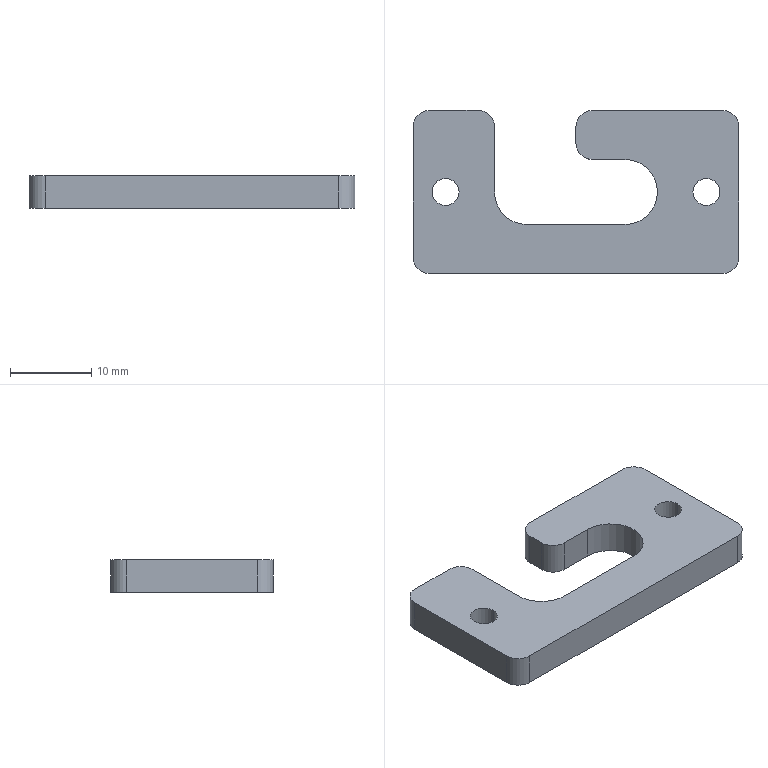Part | SolidWorks | features BreakCorner 1, FlatPattern 1, HoleWzd 1, ICE 1, SMBaseFlange 1, SheetMetal 1 | 1 solid | 24 faces | box 40 x 20 x 4 mm | volume 2269 mm3 | cylinder 13 | plane 11 | commonest cylinder face diameters 4 x7 3.3 x4 8 x2
STEP:
#1=CARTESIAN_POINT('',(-17.65,0.,-4.));
#2=VERTEX_POINT('',#1);
#3=CARTESIAN_POINT('',(-14.35,0.,-4.));
#4=VERTEX_POINT('',#3);
#5=CARTESIAN_POINT('',(-16.,0.,-4.));
#6=DIRECTION('',(0.,0.,1.));
#7=DIRECTION('',(1.,0.,0.));
#8=AXIS2_PLACEMENT_3D('',#5,#6,#7);
#9=CIRCLE('',#8,1.65);
#10=EDGE_CURVE('',#2,#4,#9,.T.);
#11=ORIENTED_EDGE('',*,*,#10,.F.);
#12=CARTESIAN_POINT('',(-17.65,0.,0.));
#13=VERTEX_POINT('',#12);
#14=CARTESIAN_POINT('',(-17.65,0.,0.));
#15=DIRECTION('',(0.,0.,1.));
#16=VECTOR('',#15,1000.);
#17=LINE('',#14,#16);
#18=EDGE_CURVE('',#2,#13,#17,.T.);
#19=ORIENTED_EDGE('',*,*,#18,.T.);
#20=CARTESIAN_POINT('',(-14.35,0.,0.));
#21=VERTEX_POINT('',#20);
#22=CARTESIAN_POINT('',(-16.,0.,0.));
#23=DIRECTION('',(0.,0.,1.));
#24=DIRECTION('',(1.,0.,0.));
#25=AXIS2_PLACEMENT_3D('',#22,#23,#24);
#26=CIRCLE('',#25,1.65);
#27=EDGE_CURVE('',#13,#21,#26,.T.);
#28=ORIENTED_EDGE('',*,*,#27,.T.);
#29=CARTESIAN_POINT('',(-14.35,0.,0.));
#30=DIRECTION('',(0.,0.,1.));
#31=VECTOR('',#30,1000.);
#32=LINE('',#29,#31);
#33=EDGE_CURVE('',#4,#21,#32,.T.);
#34=ORIENTED_EDGE('',*,*,#33,.F.);
#35=EDGE_LOOP('',(#11,#19,#28,#34));
#36=FACE_OUTER_BOUND('',#35,.T.);
#37=CARTESIAN_POINT('',(-16.,0.,0.));
#38=DIRECTION('',(0.,0.,1.));
#39=DIRECTION('',(1.,0.,0.));
#40=AXIS2_PLACEMENT_3D('',#37,#38,#39);
#41=CYLINDRICAL_SURFACE('',#40,1.65);
#42=ADVANCED_FACE('',(#36),#41,.F.);
#43=CARTESIAN_POINT('',(14.35,0.,-4.));
#44=VERTEX_POINT('',#43);
#45=CARTESIAN_POINT('',(17.65,0.,-4.));
#46=VERTEX_POINT('',#45);
#47=CARTESIAN_POINT('',(16.,0.,-4.));
#48=DIRECTION('',(0.,0.,1.));
#49=DIRECTION('',(1.,0.,0.));
#50=AXIS2_PLACEMENT_3D('',#47,#48,#49);
#51=CIRCLE('',#50,1.65);
#52=EDGE_CURVE('',#44,#46,#51,.T.);
#53=ORIENTED_EDGE('',*,*,#52,.F.);
#54=CARTESIAN_POINT('',(14.35,0.,0.));
#55=VERTEX_POINT('',#54);
#56=CARTESIAN_POINT('',(14.35,0.,0.));
#57=DIRECTION('',(0.,0.,1.));
#58=VECTOR('',#57,1000.);
#59=LINE('',#56,#58);
#60=EDGE_CURVE('',#44,#55,#59,.T.);
#61=ORIENTED_EDGE('',*,*,#60,.T.);
#62=CARTESIAN_POINT('',(17.65,0.,0.));
#63=VERTEX_POINT('',#62);
#64=CARTESIAN_POINT('',(16.,0.,0.));
#65=DIRECTION('',(0.,0.,1.));
#66=DIRECTION('',(1.,0.,0.));
#67=AXIS2_PLACEMENT_3D('',#64,#65,#66);
#68=CIRCLE('',#67,1.65);
#69=EDGE_CURVE('',#55,#63,#68,.T.);
#70=ORIENTED_EDGE('',*,*,#69,.T.);
#71=CARTESIAN_POINT('',(17.65,0.,0.));
#72=DIRECTION('',(0.,0.,1.));
#73=VECTOR('',#72,1000.);
#74=LINE('',#71,#73);
#75=EDGE_CURVE('',#46,#63,#74,.T.);
#76=ORIENTED_EDGE('',*,*,#75,.F.);
#77=EDGE_LOOP('',(#53,#61,#70,#76));
#78=FACE_OUTER_BOUND('',#77,.T.);
#79=CARTESIAN_POINT('',(16.,0.,0.));
#80=DIRECTION('',(0.,0.,1.));
#81=DIRECTION('',(1.,0.,0.));
#82=AXIS2_PLACEMENT_3D('',#79,#80,#81);
#83=CYLINDRICAL_SURFACE('',#82,1.65);
#84=ADVANCED_FACE('',(#78),#83,.F.);
#85=CARTESIAN_POINT('',(-12.,10.,-4.));
#86=VERTEX_POINT('',#85);
#87=CARTESIAN_POINT('',(-18.,10.,-4.));
#88=VERTEX_POINT('',#87);
#89=CARTESIAN_POINT('',(-20.,10.,-4.));
#90=DIRECTION('',(-1.,0.,0.));
#91=VECTOR('',#90,1000.);
#92=LINE('',#89,#91);
#93=EDGE_CURVE('',#86,#88,#92,.T.);
#94=ORIENTED_EDGE('',*,*,#93,.T.);
#95=CARTESIAN_POINT('',(-18.,10.,0.));
#96=VERTEX_POINT('',#95);
#97=CARTESIAN_POINT('',(-18.,10.,-4.));
#98=DIRECTION('',(0.,0.,1.));
#99=VECTOR('',#98,1000.);
#100=LINE('',#97,#99);
#101=EDGE_CURVE('',#88,#96,#100,.T.);
#102=ORIENTED_EDGE('',*,*,#101,.T.);
#103=CARTESIAN_POINT('',(-12.,10.,0.));
#104=VERTEX_POINT('',#103);
#105=CARTESIAN_POINT('',(-20.,10.,0.));
#106=DIRECTION('',(-1.,0.,0.));
#107=VECTOR('',#106,1000.);
#108=LINE('',#105,#107);
#109=EDGE_CURVE('',#104,#96,#108,.T.);
#110=ORIENTED_EDGE('',*,*,#109,.F.);
#111=CARTESIAN_POINT('',(-12.,10.,-4.));
#112=DIRECTION('',(0.,0.,-1.));
#113=VECTOR('',#112,1000.);
#114=LINE('',#111,#113);
#115=EDGE_CURVE('',#104,#86,#114,.T.);
#116=ORIENTED_EDGE('',*,*,#115,.T.);
#117=EDGE_LOOP('',(#94,#102,#110,#116));
#118=FACE_OUTER_BOUND('',#117,.T.);
#119=CARTESIAN_POINT('',(-20.,10.,-4.));
#120=DIRECTION('',(0.,1.,0.));
#121=DIRECTION('',(0.,0.,1.));
#122=AXIS2_PLACEMENT_3D('',#119,#120,#121);
#123=PLANE('',#122);
#124=ADVANCED_FACE('',(#118),#123,.T.);
#125=CARTESIAN_POINT('',(20.,-8.,-4.));
#126=VERTEX_POINT('',#125);
#127=CARTESIAN_POINT('',(20.,8.,-4.));
#128=VERTEX_POINT('',#127);
#129=CARTESIAN_POINT('',(20.,10.,-4.));
#130=DIRECTION('',(0.,1.,0.));
#131=VECTOR('',#130,1000.);
#132=LINE('',#129,#131);
#133=EDGE_CURVE('',#126,#128,#132,.T.);
#134=ORIENTED_EDGE('',*,*,#133,.T.);
#135=CARTESIAN_POINT('',(20.,8.,0.));
#136=VERTEX_POINT('',#135);
#137=CARTESIAN_POINT('',(20.,8.,-4.));
#138=DIRECTION('',(0.,0.,1.));
#139=VECTOR('',#138,1000.);
#140=LINE('',#137,#139);
#141=EDGE_CURVE('',#128,#136,#140,.T.);
#142=ORIENTED_EDGE('',*,*,#141,.T.);
#143=CARTESIAN_POINT('',(20.,-8.,0.));
#144=VERTEX_POINT('',#143);
#145=CARTESIAN_POINT('',(20.,10.,0.));
#146=DIRECTION('',(0.,1.,0.));
#147=VECTOR('',#146,1000.);
#148=LINE('',#145,#147);
#149=EDGE_CURVE('',#144,#136,#148,.T.);
#150=ORIENTED_EDGE('',*,*,#149,.F.);
#151=CARTESIAN_POINT('',(20.,-8.,-4.));
#152=DIRECTION('',(0.,0.,-1.));
#153=VECTOR('',#152,1000.);
#154=LINE('',#151,#153);
#155=EDGE_CURVE('',#144,#126,#154,.T.);
#156=ORIENTED_EDGE('',*,*,#155,.T.);
#157=EDGE_LOOP('',(#134,#142,#150,#156));
#158=FACE_OUTER_BOUND('',#157,.T.);
#159=CARTESIAN_POINT('',(20.,10.,-4.));
#160=DIRECTION('',(1.,0.,0.));
#161=DIRECTION('',(0.,1.,0.));
#162=AXIS2_PLACEMENT_3D('',#159,#160,#161);
#163=PLANE('',#162);
#164=ADVANCED_FACE('',(#158),#163,.T.);
#165=CARTESIAN_POINT('',(-18.,-10.,-4.));
#166=VERTEX_POINT('',#165);
#167=CARTESIAN_POINT('',(18.,-10.,-4.));
#168=VERTEX_POINT('',#167);
#169=CARTESIAN_POINT('',(-20.,-10.,-4.));
#170=DIRECTION('',(1.,0.,0.));
#171=VECTOR('',#170,1000.);
#172=LINE('',#169,#171);
#173=EDGE_CURVE('',#166,#168,#172,.T.);
#174=ORIENTED_EDGE('',*,*,#173,.T.);
#175=CARTESIAN_POINT('',(18.,-10.,0.));
#176=VERTEX_POINT('',#175);
#177=CARTESIAN_POINT('',(18.,-10.,-4.));
#178=DIRECTION('',(0.,0.,1.));
#179=VECTOR('',#178,1000.);
#180=LINE('',#177,#179);
#181=EDGE_CURVE('',#168,#176,#180,.T.);
#182=ORIENTED_EDGE('',*,*,#181,.T.);
#183=CARTESIAN_POINT('',(-18.,-10.,0.));
#184=VERTEX_POINT('',#183);
#185=CARTESIAN_POINT('',(-20.,-10.,0.));
#186=DIRECTION('',(1.,0.,0.));
#187=VECTOR('',#186,1000.);
#188=LINE('',#185,#187);
#189=EDGE_CURVE('',#184,#176,#188,.T.);
#190=ORIENTED_EDGE('',*,*,#189,.F.);
#191=CARTESIAN_POINT('',(-18.,-10.,-4.));
#192=DIRECTION('',(0.,0.,-1.));
#193=VECTOR('',#192,1000.);
#194=LINE('',#191,#193);
#195=EDGE_CURVE('',#184,#166,#194,.T.);
#196=ORIENTED_EDGE('',*,*,#195,.T.);
#197=EDGE_LOOP('',(#174,#182,#190,#196));
#198=FACE_OUTER_BOUND('',#197,.T.);
#199=CARTESIAN_POINT('',(-20.,-10.,-4.));
#200=DIRECTION('',(0.,-1.,0.));
#201=DIRECTION('',(0.,0.,-1.));
#202=AXIS2_PLACEMENT_3D('',#199,#200,#201);
#203=PLANE('',#202);
#204=ADVANCED_FACE('',(#198),#203,.T.);
#205=CARTESIAN_POINT('',(-20.,8.,-4.));
#206=VERTEX_POINT('',#205);
#207=CARTESIAN_POINT('',(-20.,-8.,-4.));
#208=VERTEX_POINT('',#207);
#209=CARTESIAN_POINT('',(-20.,10.,-4.));
#210=DIRECTION('',(0.,-1.,0.));
#211=VECTOR('',#210,1000.);
#212=LINE('',#209,#211);
#213=EDGE_CURVE('',#206,#208,#212,.T.);
#214=ORIENTED_EDGE('',*,*,#213,.T.);
#215=CARTESIAN_POINT('',(-20.,-8.,0.));
#216=VERTEX_POINT('',#215);
#217=CARTESIAN_POINT('',(-20.,-8.,-4.));
#218=DIRECTION('',(0.,0.,1.));
#219=VECTOR('',#218,1000.);
#220=LINE('',#217,#219);
#221=EDGE_CURVE('',#208,#216,#220,.T.);
#222=ORIENTED_EDGE('',*,*,#221,.T.);
#223=CARTESIAN_POINT('',(-20.,8.,0.));
#224=VERTEX_POINT('',#223);
#225=CARTESIAN_POINT('',(-20.,10.,0.));
#226=DIRECTION('',(0.,-1.,0.));
#227=VECTOR('',#226,1000.);
#228=LINE('',#225,#227);
#229=EDGE_CURVE('',#224,#216,#228,.T.);
#230=ORIENTED_EDGE('',*,*,#229,.F.);
#231=CARTESIAN_POINT('',(-20.,8.,-4.));
#232=DIRECTION('',(0.,0.,-1.));
#233=VECTOR('',#232,1000.);
#234=LINE('',#231,#233);
#235=EDGE_CURVE('',#224,#206,#234,.T.);
#236=ORIENTED_EDGE('',*,*,#235,.T.);
#237=EDGE_LOOP('',(#214,#222,#230,#236));
#238=FACE_OUTER_BOUND('',#237,.T.);
#239=CARTESIAN_POINT('',(-20.,10.,-4.));
#240=DIRECTION('',(-1.,0.,0.));
#241=DIRECTION('',(0.,0.,1.));
#242=AXIS2_PLACEMENT_3D('',#239,#240,#241);
#243=PLANE('',#242);
#244=ADVANCED_FACE('',(#238),#243,.T.);
#245=CARTESIAN_POINT('',(18.,10.,-4.));
#246=VERTEX_POINT('',#245);
#247=CARTESIAN_POINT('',(2.,10.,-4.));
#248=VERTEX_POINT('',#247);
#249=CARTESIAN_POINT('',(-20.,10.,-4.));
#250=DIRECTION('',(-1.,0.,0.));
#251=VECTOR('',#250,1000.);
#252=LINE('',#249,#251);
#253=EDGE_CURVE('',#246,#248,#252,.T.);
#254=ORIENTED_EDGE('',*,*,#253,.T.);
#255=CARTESIAN_POINT('',(2.,10.,0.));
#256=VERTEX_POINT('',#255);
#257=CARTESIAN_POINT('',(2.,10.,0.));
#258=DIRECTION('',(0.,0.,1.));
#259=VECTOR('',#258,1000.);
#260=LINE('',#257,#259);
#261=EDGE_CURVE('',#248,#256,#260,.T.);
#262=ORIENTED_EDGE('',*,*,#261,.T.);
#263=CARTESIAN_POINT('',(18.,10.,0.));
#264=VERTEX_POINT('',#263);
#265=CARTESIAN_POINT('',(-20.,10.,0.));
#266=DIRECTION('',(-1.,0.,0.));
#267=VECTOR('',#266,1000.);
#268=LINE('',#265,#267);
#269=EDGE_CURVE('',#264,#256,#268,.T.);
#270=ORIENTED_EDGE('',*,*,#269,.F.);
#271=CARTESIAN_POINT('',(18.,10.,-4.));
#272=DIRECTION('',(0.,0.,-1.));
#273=VECTOR('',#272,1000.);
#274=LINE('',#271,#273);
#275=EDGE_CURVE('',#264,#246,#274,.T.);
#276=ORIENTED_EDGE('',*,*,#275,.T.);
#277=EDGE_LOOP('',(#254,#262,#270,#276));
#278=FACE_OUTER_BOUND('',#277,.T.);
#279=CARTESIAN_POINT('',(-20.,10.,-4.));
#280=DIRECTION('',(0.,1.,0.));
#281=DIRECTION('',(0.,0.,1.));
#282=AXIS2_PLACEMENT_3D('',#279,#280,#281);
#283=PLANE('',#282);
#284=ADVANCED_FACE('',(#278),#283,.T.);
#285=CARTESIAN_POINT('',(-16.,0.,-4.));
#286=DIRECTION('',(0.,0.,1.));
#287=DIRECTION('',(1.,0.,0.));
#288=AXIS2_PLACEMENT_3D('',#285,#286,#287);
#289=CIRCLE('',#288,1.65);
#290=EDGE_CURVE('',#4,#2,#289,.T.);
#291=ORIENTED_EDGE('',*,*,#290,.T.);
#292=ORIENTED_EDGE('',*,*,#10,.T.);
#293=EDGE_LOOP('',(#291,#292));
#294=FACE_BOUND('',#293,.T.);
#295=CARTESIAN_POINT('',(16.,0.,-4.));
#296=DIRECTION('',(0.,0.,1.));
#297=DIRECTION('',(1.,0.,0.));
#298=AXIS2_PLACEMENT_3D('',#295,#296,#297);
#299=CIRCLE('',#298,1.65);
#300=EDGE_CURVE('',#46,#44,#299,.T.);
#301=ORIENTED_EDGE('',*,*,#300,.T.);
#302=ORIENTED_EDGE('',*,*,#52,.T.);
#303=EDGE_LOOP('',(#301,#302));
#304=FACE_BOUND('',#303,.T.);
#305=CARTESIAN_POINT('',(6.,4.,-4.));
#306=VERTEX_POINT('',#305);
#307=CARTESIAN_POINT('',(2.,4.,-4.));
#308=VERTEX_POINT('',#307);
#309=CARTESIAN_POINT('',(0.,4.,-4.));
#310=DIRECTION('',(-1.,0.,0.));
#311=VECTOR('',#310,1000.);
#312=LINE('',#309,#311);
#313=EDGE_CURVE('',#306,#308,#312,.T.);
#314=ORIENTED_EDGE('',*,*,#313,.T.);
#315=CARTESIAN_POINT('',(0.,6.,-4.));
#316=VERTEX_POINT('',#315);
#317=CARTESIAN_POINT('',(2.,6.,-4.));
#318=DIRECTION('',(0.,0.,-1.));
#319=DIRECTION('',(1.,0.,0.));
#320=AXIS2_PLACEMENT_3D('',#317,#318,#319);
#321=CIRCLE('',#320,2.);
#322=EDGE_CURVE('',#308,#316,#321,.T.);
#323=ORIENTED_EDGE('',*,*,#322,.T.);
#324=CARTESIAN_POINT('',(0.,8.,-4.));
#325=VERTEX_POINT('',#324);
#326=CARTESIAN_POINT('',(0.,0.,-4.));
#327=DIRECTION('',(0.,1.,0.));
#328=VECTOR('',#327,1000.);
#329=LINE('',#326,#328);
#330=EDGE_CURVE('',#316,#325,#329,.T.);
#331=ORIENTED_EDGE('',*,*,#330,.T.);
#332=CARTESIAN_POINT('',(2.,8.,-4.));
#333=DIRECTION('',(0.,0.,-1.));
#334=DIRECTION('',(1.,0.,0.));
#335=AXIS2_PLACEMENT_3D('',#332,#333,#334);
#336=CIRCLE('',#335,2.);
#337=EDGE_CURVE('',#325,#248,#336,.T.);
#338=ORIENTED_EDGE('',*,*,#337,.T.);
#339=ORIENTED_EDGE('',*,*,#253,.F.);
#340=CARTESIAN_POINT('',(18.,8.,-4.));
#341=DIRECTION('',(0.,0.,-1.));
#342=DIRECTION('',(1.,0.,0.));
#343=AXIS2_PLACEMENT_3D('',#340,#341,#342);
#344=CIRCLE('',#343,2.);
#345=EDGE_CURVE('',#246,#128,#344,.T.);
#346=ORIENTED_EDGE('',*,*,#345,.T.);
#347=ORIENTED_EDGE('',*,*,#133,.F.);
#348=CARTESIAN_POINT('',(18.,-8.,-4.));
#349=DIRECTION('',(0.,0.,-1.));
#350=DIRECTION('',(1.,0.,0.));
#351=AXIS2_PLACEMENT_3D('',#348,#349,#350);
#352=CIRCLE('',#351,2.);
#353=EDGE_CURVE('',#126,#168,#352,.T.);
#354=ORIENTED_EDGE('',*,*,#353,.T.);
#355=ORIENTED_EDGE('',*,*,#173,.F.);
#356=CARTESIAN_POINT('',(-18.,-8.,-4.));
#357=DIRECTION('',(0.,0.,-1.));
#358=DIRECTION('',(1.,0.,0.));
#359=AXIS2_PLACEMENT_3D('',#356,#357,#358);
#360=CIRCLE('',#359,2.);
#361=EDGE_CURVE('',#166,#208,#360,.T.);
#362=ORIENTED_EDGE('',*,*,#361,.T.);
#363=ORIENTED_EDGE('',*,*,#213,.F.);
#364=CARTESIAN_POINT('',(-18.,8.,-4.));
#365=DIRECTION('',(0.,0.,-1.));
#366=DIRECTION('',(1.,0.,0.));
#367=AXIS2_PLACEMENT_3D('',#364,#365,#366);
#368=CIRCLE('',#367,2.);
#369=EDGE_CURVE('',#206,#88,#368,.T.);
#370=ORIENTED_EDGE('',*,*,#369,.T.);
#371=ORIENTED_EDGE('',*,*,#93,.F.);
#372=CARTESIAN_POINT('',(-10.,8.,-4.));
#373=VERTEX_POINT('',#372);
#374=CARTESIAN_POINT('',(-12.,8.,-4.));
#375=DIRECTION('',(0.,0.,-1.));
#376=DIRECTION('',(1.,0.,0.));
#377=AXIS2_PLACEMENT_3D('',#374,#375,#376);
#378=CIRCLE('',#377,2.);
#379=EDGE_CURVE('',#86,#373,#378,.T.);
#380=ORIENTED_EDGE('',*,*,#379,.T.);
#381=CARTESIAN_POINT('',(-10.,0.,-4.));
#382=VERTEX_POINT('',#381);
#383=CARTESIAN_POINT('',(-10.,0.,-4.));
#384=DIRECTION('',(0.,-1.,0.));
#385=VECTOR('',#384,1000.);
#386=LINE('',#383,#385);
#387=EDGE_CURVE('',#373,#382,#386,.T.);
#388=ORIENTED_EDGE('',*,*,#387,.T.);
#389=CARTESIAN_POINT('',(-6.,-4.,-4.));
#390=VERTEX_POINT('',#389);
#391=CARTESIAN_POINT('',(-6.,0.,-4.));
#392=DIRECTION('',(0.,0.,1.));
#393=DIRECTION('',(1.,0.,0.));
#394=AXIS2_PLACEMENT_3D('',#391,#392,#393);
#395=CIRCLE('',#394,4.);
#396=EDGE_CURVE('',#382,#390,#395,.T.);
#397=ORIENTED_EDGE('',*,*,#396,.T.);
#398=CARTESIAN_POINT('',(6.,-4.,-4.));
#399=VERTEX_POINT('',#398);
#400=CARTESIAN_POINT('',(0.,-4.,-4.));
#401=DIRECTION('',(1.,0.,0.));
#402=VECTOR('',#401,1000.);
#403=LINE('',#400,#402);
#404=EDGE_CURVE('',#390,#399,#403,.T.);
#405=ORIENTED_EDGE('',*,*,#404,.T.);
#406=CARTESIAN_POINT('',(6.,0.,-4.));
#407=DIRECTION('',(0.,0.,1.));
#408=DIRECTION('',(1.,0.,0.));
#409=AXIS2_PLACEMENT_3D('',#406,#407,#408);
#410=CIRCLE('',#409,4.);
#411=EDGE_CURVE('',#399,#306,#410,.T.);
#412=ORIENTED_EDGE('',*,*,#411,.T.);
#413=EDGE_LOOP('',(#314,#323,#331,#338,#339,#346,#347,#354,#355,#362,#363,#370,#371,#380,#388,#397,#405,#412));
#414=FACE_OUTER_BOUND('',#413,.T.);
#415=CARTESIAN_POINT('',(0.,0.,-4.));
#416=DIRECTION('',(0.,0.,1.));
#417=DIRECTION('',(1.,0.,0.));
#418=AXIS2_PLACEMENT_3D('',#415,#416,#417);
#419=PLANE('',#418);
#420=ADVANCED_FACE('',(#294,#304,#414),#419,.F.);
#421=CARTESIAN_POINT('',(-16.,0.,0.));
#422=DIRECTION('',(0.,0.,1.));
#423=DIRECTION('',(1.,0.,0.));
#424=AXIS2_PLACEMENT_3D('',#421,#422,#423);
#425=CIRCLE('',#424,1.65);
#426=EDGE_CURVE('',#21,#13,#425,.T.);
#427=ORIENTED_EDGE('',*,*,#426,.F.);
#428=ORIENTED_EDGE('',*,*,#27,.F.);
#429=EDGE_LOOP('',(#427,#428));
#430=FACE_BOUND('',#429,.T.);
#431=CARTESIAN_POINT('',(16.,0.,0.));
#432=DIRECTION('',(0.,0.,1.));
#433=DIRECTION('',(1.,0.,0.));
#434=AXIS2_PLACEMENT_3D('',#431,#432,#433);
#435=CIRCLE('',#434,1.65);
#436=EDGE_CURVE('',#63,#55,#435,.T.);
#437=ORIENTED_EDGE('',*,*,#436,.F.);
#438=ORIENTED_EDGE('',*,*,#69,.F.);
#439=EDGE_LOOP('',(#437,#438));
#440=FACE_BOUND('',#439,.T.);
#441=CARTESIAN_POINT('',(0.,6.,0.));
#442=VERTEX_POINT('',#441);
#443=CARTESIAN_POINT('',(0.,8.,0.));
#444=VERTEX_POINT('',#443);
#445=CARTESIAN_POINT('',(0.,0.,0.));
#446=DIRECTION('',(0.,1.,0.));
#447=VECTOR('',#446,1000.);
#448=LINE('',#445,#447);
#449=EDGE_CURVE('',#442,#444,#448,.T.);
#450=ORIENTED_EDGE('',*,*,#449,.F.);
#451=CARTESIAN_POINT('',(2.,4.,0.));
#452=VERTEX_POINT('',#451);
#453=CARTESIAN_POINT('',(2.,6.,0.));
#454=DIRECTION('',(0.,0.,1.));
#455=DIRECTION('',(1.,0.,0.));
#456=AXIS2_PLACEMENT_3D('',#453,#454,#455);
#457=CIRCLE('',#456,2.);
#458=EDGE_CURVE('',#442,#452,#457,.T.);
#459=ORIENTED_EDGE('',*,*,#458,.T.);
#460=CARTESIAN_POINT('',(6.,4.,0.));
#461=VERTEX_POINT('',#460);
#462=CARTESIAN_POINT('',(0.,4.,0.));
#463=DIRECTION('',(-1.,0.,0.));
#464=VECTOR('',#463,1000.);
#465=LINE('',#462,#464);
#466=EDGE_CURVE('',#461,#452,#465,.T.);
#467=ORIENTED_EDGE('',*,*,#466,.F.);
#468=CARTESIAN_POINT('',(6.,-4.,0.));
#469=VERTEX_POINT('',#468);
#470=CARTESIAN_POINT('',(6.,0.,0.));
#471=DIRECTION('',(0.,0.,1.));
#472=DIRECTION('',(1.,0.,0.));
#473=AXIS2_PLACEMENT_3D('',#470,#471,#472);
#474=CIRCLE('',#473,4.);
#475=EDGE_CURVE('',#469,#461,#474,.T.);
#476=ORIENTED_EDGE('',*,*,#475,.F.);
#477=CARTESIAN_POINT('',(-6.,-4.,0.));
#478=VERTEX_POINT('',#477);
#479=CARTESIAN_POINT('',(0.,-4.,0.));
#480=DIRECTION('',(1.,0.,0.));
#481=VECTOR('',#480,1000.);
#482=LINE('',#479,#481);
#483=EDGE_CURVE('',#478,#469,#482,.T.);
#484=ORIENTED_EDGE('',*,*,#483,.F.);
#485=CARTESIAN_POINT('',(-10.,0.,0.));
#486=VERTEX_POINT('',#485);
#487=CARTESIAN_POINT('',(-6.,0.,0.));
#488=DIRECTION('',(0.,0.,1.));
#489=DIRECTION('',(1.,0.,0.));
#490=AXIS2_PLACEMENT_3D('',#487,#488,#489);
#491=CIRCLE('',#490,4.);
#492=EDGE_CURVE('',#486,#478,#491,.T.);
#493=ORIENTED_EDGE('',*,*,#492,.F.);
#494=CARTESIAN_POINT('',(-10.,8.,0.));
#495=VERTEX_POINT('',#494);
#496=CARTESIAN_POINT('',(-10.,0.,0.));
#497=DIRECTION('',(0.,-1.,0.));
#498=VECTOR('',#497,1000.);
#499=LINE('',#496,#498);
#500=EDGE_CURVE('',#495,#486,#499,.T.);
#501=ORIENTED_EDGE('',*,*,#500,.F.);
#502=CARTESIAN_POINT('',(-12.,8.,0.));
#503=DIRECTION('',(0.,0.,1.));
#504=DIRECTION('',(1.,0.,0.));
#505=AXIS2_PLACEMENT_3D('',#502,#503,#504);
#506=CIRCLE('',#505,2.);
#507=EDGE_CURVE('',#495,#104,#506,.T.);
#508=ORIENTED_EDGE('',*,*,#507,.T.);
#509=ORIENTED_EDGE('',*,*,#109,.T.);
#510=CARTESIAN_POINT('',(-18.,8.,0.));
#511=DIRECTION('',(0.,0.,1.));
#512=DIRECTION('',(1.,0.,0.));
#513=AXIS2_PLACEMENT_3D('',#510,#511,#512);
#514=CIRCLE('',#513,2.);
#515=EDGE_CURVE('',#96,#224,#514,.T.);
#516=ORIENTED_EDGE('',*,*,#515,.T.);
#517=ORIENTED_EDGE('',*,*,#229,.T.);
#518=CARTESIAN_POINT('',(-18.,-8.,0.));
#519=DIRECTION('',(0.,0.,1.));
#520=DIRECTION('',(1.,0.,0.));
#521=AXIS2_PLACEMENT_3D('',#518,#519,#520);
#522=CIRCLE('',#521,2.);
#523=EDGE_CURVE('',#216,#184,#522,.T.);
#524=ORIENTED_EDGE('',*,*,#523,.T.);
#525=ORIENTED_EDGE('',*,*,#189,.T.);
#526=CARTESIAN_POINT('',(18.,-8.,0.));
#527=DIRECTION('',(0.,0.,1.));
#528=DIRECTION('',(1.,0.,0.));
#529=AXIS2_PLACEMENT_3D('',#526,#527,#528);
#530=CIRCLE('',#529,2.);
#531=EDGE_CURVE('',#176,#144,#530,.T.);
#532=ORIENTED_EDGE('',*,*,#531,.T.);
#533=ORIENTED_EDGE('',*,*,#149,.T.);
#534=CARTESIAN_POINT('',(18.,8.,0.));
#535=DIRECTION('',(0.,0.,1.));
#536=DIRECTION('',(1.,0.,0.));
#537=AXIS2_PLACEMENT_3D('',#534,#535,#536);
#538=CIRCLE('',#537,2.);
#539=EDGE_CURVE('',#136,#264,#538,.T.);
#540=ORIENTED_EDGE('',*,*,#539,.T.);
#541=ORIENTED_EDGE('',*,*,#269,.T.);
#542=CARTESIAN_POINT('',(2.,8.,0.));
#543=DIRECTION('',(0.,0.,1.));
#544=DIRECTION('',(1.,0.,0.));
#545=AXIS2_PLACEMENT_3D('',#542,#543,#544);
#546=CIRCLE('',#545,2.);
#547=EDGE_CURVE('',#256,#444,#546,.T.);
#548=ORIENTED_EDGE('',*,*,#547,.T.);
#549=EDGE_LOOP('',(#450,#459,#467,#476,#484,#493,#501,#508,#509,#516,#517,#524,#525,#532,#533,#540,#541,#548));
#550=FACE_OUTER_BOUND('',#549,.T.);
#551=CARTESIAN_POINT('',(0.,0.,0.));
#552=DIRECTION('',(0.,0.,1.));
#553=DIRECTION('',(1.,0.,0.));
#554=AXIS2_PLACEMENT_3D('',#551,#552,#553);
#555=PLANE('',#554);
#556=ADVANCED_FACE('',(#430,#440,#550),#555,.T.);
#557=ORIENTED_EDGE('',*,*,#387,.F.);
#558=CARTESIAN_POINT('',(-10.,8.,0.));
#559=DIRECTION('',(0.,0.,1.));
#560=VECTOR('',#559,1000.);
#561=LINE('',#558,#560);
#562=EDGE_CURVE('',#373,#495,#561,.T.);
#563=ORIENTED_EDGE('',*,*,#562,.T.);
#564=ORIENTED_EDGE('',*,*,#500,.T.);
#565=CARTESIAN_POINT('',(-10.,0.,56.125));
#566=DIRECTION('',(0.,0.,-1.));
#567=VECTOR('',#566,1000.);
#568=LINE('',#565,#567);
#569=EDGE_CURVE('',#486,#382,#568,.T.);
#570=ORIENTED_EDGE('',*,*,#569,.T.);
#571=EDGE_LOOP('',(#557,#563,#564,#570));
#572=FACE_OUTER_BOUND('',#571,.T.);
#573=CARTESIAN_POINT('',(-10.,0.,56.125));
#574=DIRECTION('',(-1.,0.,0.));
#575=DIRECTION('',(0.,0.,1.));
#576=AXIS2_PLACEMENT_3D('',#573,#574,#575);
#577=PLANE('',#576);
#578=ADVANCED_FACE('',(#572),#577,.F.);
#579=ORIENTED_EDGE('',*,*,#396,.F.);
#580=ORIENTED_EDGE('',*,*,#569,.F.);
#581=ORIENTED_EDGE('',*,*,#492,.T.);
#582=CARTESIAN_POINT('',(-6.,-4.,56.125));
#583=DIRECTION('',(0.,0.,-1.));
#584=VECTOR('',#583,1000.);
#585=LINE('',#582,#584);
#586=EDGE_CURVE('',#478,#390,#585,.T.);
#587=ORIENTED_EDGE('',*,*,#586,.T.);
#588=EDGE_LOOP('',(#579,#580,#581,#587));
#589=FACE_OUTER_BOUND('',#588,.T.);
#590=CARTESIAN_POINT('',(-6.,0.,56.125));
#591=DIRECTION('',(0.,0.,-1.));
#592=DIRECTION('',(-1.,0.,0.));
#593=AXIS2_PLACEMENT_3D('',#590,#591,#592);
#594=CYLINDRICAL_SURFACE('',#593,4.);
#595=ADVANCED_FACE('',(#589),#594,.F.);
#596=ORIENTED_EDGE('',*,*,#404,.F.);
#597=ORIENTED_EDGE('',*,*,#586,.F.);
#598=ORIENTED_EDGE('',*,*,#483,.T.);
#599=CARTESIAN_POINT('',(6.,-4.,56.125));
#600=DIRECTION('',(0.,0.,-1.));
#601=VECTOR('',#600,1000.);
#602=LINE('',#599,#601);
#603=EDGE_CURVE('',#469,#399,#602,.T.);
#604=ORIENTED_EDGE('',*,*,#603,.T.);
#605=EDGE_LOOP('',(#596,#597,#598,#604));
#606=FACE_OUTER_BOUND('',#605,.T.);
#607=CARTESIAN_POINT('',(-6.,-4.,56.125));
#608=DIRECTION('',(0.,-1.,0.));
#609=DIRECTION('',(1.,0.,0.));
#610=AXIS2_PLACEMENT_3D('',#607,#608,#609);
#611=PLANE('',#610);
#612=ADVANCED_FACE('',(#606),#611,.F.);
#613=ORIENTED_EDGE('',*,*,#411,.F.);
#614=ORIENTED_EDGE('',*,*,#603,.F.);
#615=ORIENTED_EDGE('',*,*,#475,.T.);
#616=CARTESIAN_POINT('',(6.,4.,56.125));
#617=DIRECTION('',(0.,0.,-1.));
#618=VECTOR('',#617,1000.);
#619=LINE('',#616,#618);
#620=EDGE_CURVE('',#461,#306,#619,.T.);
#621=ORIENTED_EDGE('',*,*,#620,.T.);
#622=EDGE_LOOP('',(#613,#614,#615,#621));
#623=FACE_OUTER_BOUND('',#622,.T.);
#624=CARTESIAN_POINT('',(6.,0.,56.125));
#625=DIRECTION('',(0.,0.,-1.));
#626=DIRECTION('',(-1.,0.,0.));
#627=AXIS2_PLACEMENT_3D('',#624,#625,#626);
#628=CYLINDRICAL_SURFACE('',#627,4.);
#629=ADVANCED_FACE('',(#623),#628,.F.);
#630=ORIENTED_EDGE('',*,*,#466,.T.);
#631=CARTESIAN_POINT('',(2.,4.,56.125));
#632=DIRECTION('',(0.,0.,-1.));
#633=VECTOR('',#632,1000.);
#634=LINE('',#631,#633);
#635=EDGE_CURVE('',#452,#308,#634,.T.);
#636=ORIENTED_EDGE('',*,*,#635,.T.);
#637=ORIENTED_EDGE('',*,*,#313,.F.);
#638=ORIENTED_EDGE('',*,*,#620,.F.);
#639=EDGE_LOOP('',(#630,#636,#637,#638));
#640=FACE_OUTER_BOUND('',#639,.T.);
#641=CARTESIAN_POINT('',(0.,4.,56.125));
#642=DIRECTION('',(0.,1.,0.));
#643=DIRECTION('',(-1.,0.,0.));
#644=AXIS2_PLACEMENT_3D('',#641,#642,#643);
#645=PLANE('',#644);
#646=ADVANCED_FACE('',(#640),#645,.F.);
#647=ORIENTED_EDGE('',*,*,#330,.F.);
#648=CARTESIAN_POINT('',(0.,6.,56.125));
#649=DIRECTION('',(0.,0.,1.));
#650=VECTOR('',#649,1000.);
#651=LINE('',#648,#650);
#652=EDGE_CURVE('',#316,#442,#651,.T.);
#653=ORIENTED_EDGE('',*,*,#652,.T.);
#654=ORIENTED_EDGE('',*,*,#449,.T.);
#655=CARTESIAN_POINT('',(0.,8.,-4.));
#656=DIRECTION('',(0.,0.,-1.));
#657=VECTOR('',#656,1000.);
#658=LINE('',#655,#657);
#659=EDGE_CURVE('',#444,#325,#658,.T.);
#660=ORIENTED_EDGE('',*,*,#659,.T.);
#661=EDGE_LOOP('',(#647,#653,#654,#660));
#662=FACE_OUTER_BOUND('',#661,.T.);
#663=CARTESIAN_POINT('',(0.,12.71,56.125));
#664=DIRECTION('',(1.,0.,0.));
#665=DIRECTION('',(0.,1.,0.));
#666=AXIS2_PLACEMENT_3D('',#663,#664,#665);
#667=PLANE('',#666);
#668=ADVANCED_FACE('',(#662),#667,.F.);
#669=ORIENTED_EDGE('',*,*,#458,.F.);
#670=ORIENTED_EDGE('',*,*,#652,.F.);
#671=ORIENTED_EDGE('',*,*,#322,.F.);
#672=ORIENTED_EDGE('',*,*,#635,.F.);
#673=EDGE_LOOP('',(#669,#670,#671,#672));
#674=FACE_OUTER_BOUND('',#673,.T.);
#675=CARTESIAN_POINT('',(2.,6.,56.125));
#676=DIRECTION('',(0.,0.,-1.));
#677=DIRECTION('',(-1.,0.,0.));
#678=AXIS2_PLACEMENT_3D('',#675,#676,#677);
#679=CYLINDRICAL_SURFACE('',#678,2.);
#680=ADVANCED_FACE('',(#674),#679,.T.);
#681=ORIENTED_EDGE('',*,*,#547,.F.);
#682=ORIENTED_EDGE('',*,*,#261,.F.);
#683=ORIENTED_EDGE('',*,*,#337,.F.);
#684=ORIENTED_EDGE('',*,*,#659,.F.);
#685=EDGE_LOOP('',(#681,#682,#683,#684));
#686=FACE_OUTER_BOUND('',#685,.T.);
#687=CARTESIAN_POINT('',(2.,8.,56.125));
#688=DIRECTION('',(0.,0.,1.));
#689=DIRECTION('',(1.,0.,0.));
#690=AXIS2_PLACEMENT_3D('',#687,#688,#689);
#691=CYLINDRICAL_SURFACE('',#690,2.);
#692=ADVANCED_FACE('',(#686),#691,.T.);
#693=ORIENTED_EDGE('',*,*,#345,.F.);
#694=ORIENTED_EDGE('',*,*,#275,.F.);
#695=ORIENTED_EDGE('',*,*,#539,.F.);
#696=ORIENTED_EDGE('',*,*,#141,.F.);
#697=EDGE_LOOP('',(#693,#694,#695,#696));
#698=FACE_OUTER_BOUND('',#697,.T.);
#699=CARTESIAN_POINT('',(18.,8.,-4.));
#700=DIRECTION('',(0.,0.,1.));
#701=DIRECTION('',(1.,0.,0.));
#702=AXIS2_PLACEMENT_3D('',#699,#700,#701);
#703=CYLINDRICAL_SURFACE('',#702,2.);
#704=ADVANCED_FACE('',(#698),#703,.T.);
#705=ORIENTED_EDGE('',*,*,#353,.F.);
#706=ORIENTED_EDGE('',*,*,#155,.F.);
#707=ORIENTED_EDGE('',*,*,#531,.F.);
#708=ORIENTED_EDGE('',*,*,#181,.F.);
#709=EDGE_LOOP('',(#705,#706,#707,#708));
#710=FACE_OUTER_BOUND('',#709,.T.);
#711=CARTESIAN_POINT('',(18.,-8.,-4.));
#712=DIRECTION('',(0.,0.,1.));
#713=DIRECTION('',(1.,0.,0.));
#714=AXIS2_PLACEMENT_3D('',#711,#712,#713);
#715=CYLINDRICAL_SURFACE('',#714,2.);
#716=ADVANCED_FACE('',(#710),#715,.T.);
#717=ORIENTED_EDGE('',*,*,#361,.F.);
#718=ORIENTED_EDGE('',*,*,#195,.F.);
#719=ORIENTED_EDGE('',*,*,#523,.F.);
#720=ORIENTED_EDGE('',*,*,#221,.F.);
#721=EDGE_LOOP('',(#717,#718,#719,#720));
#722=FACE_OUTER_BOUND('',#721,.T.);
#723=CARTESIAN_POINT('',(-18.,-8.,-4.));
#724=DIRECTION('',(0.,0.,1.));
#725=DIRECTION('',(1.,0.,0.));
#726=AXIS2_PLACEMENT_3D('',#723,#724,#725);
#727=CYLINDRICAL_SURFACE('',#726,2.);
#728=ADVANCED_FACE('',(#722),#727,.T.);
#729=ORIENTED_EDGE('',*,*,#369,.F.);
#730=ORIENTED_EDGE('',*,*,#235,.F.);
#731=ORIENTED_EDGE('',*,*,#515,.F.);
#732=ORIENTED_EDGE('',*,*,#101,.F.);
#733=EDGE_LOOP('',(#729,#730,#731,#732));
#734=FACE_OUTER_BOUND('',#733,.T.);
#735=CARTESIAN_POINT('',(-18.,8.,-4.));
#736=DIRECTION('',(0.,0.,1.));
#737=DIRECTION('',(1.,0.,0.));
#738=AXIS2_PLACEMENT_3D('',#735,#736,#737);
#739=CYLINDRICAL_SURFACE('',#738,2.);
#740=ADVANCED_FACE('',(#734),#739,.T.);
#741=ORIENTED_EDGE('',*,*,#379,.F.);
#742=ORIENTED_EDGE('',*,*,#115,.F.);
#743=ORIENTED_EDGE('',*,*,#507,.F.);
#744=ORIENTED_EDGE('',*,*,#562,.F.);
#745=EDGE_LOOP('',(#741,#742,#743,#744));
#746=FACE_OUTER_BOUND('',#745,.T.);
#747=CARTESIAN_POINT('',(-12.,8.,56.125));
#748=DIRECTION('',(0.,0.,-1.));
#749=DIRECTION('',(-1.,0.,0.));
#750=AXIS2_PLACEMENT_3D('',#747,#748,#749);
#751=CYLINDRICAL_SURFACE('',#750,2.);
#752=ADVANCED_FACE('',(#746),#751,.T.);
#753=ORIENTED_EDGE('',*,*,#60,.F.);
#754=ORIENTED_EDGE('',*,*,#300,.F.);
#755=ORIENTED_EDGE('',*,*,#75,.T.);
#756=ORIENTED_EDGE('',*,*,#436,.T.);
#757=EDGE_LOOP('',(#753,#754,#755,#756));
#758=FACE_OUTER_BOUND('',#757,.T.);
#759=CARTESIAN_POINT('',(16.,0.,0.));
#760=DIRECTION('',(0.,0.,1.));
#761=DIRECTION('',(1.,0.,0.));
#762=AXIS2_PLACEMENT_3D('',#759,#760,#761);
#763=CYLINDRICAL_SURFACE('',#762,1.65);
#764=ADVANCED_FACE('',(#758),#763,.F.);
#765=ORIENTED_EDGE('',*,*,#18,.F.);
#766=ORIENTED_EDGE('',*,*,#290,.F.);
#767=ORIENTED_EDGE('',*,*,#33,.T.);
#768=ORIENTED_EDGE('',*,*,#426,.T.);
#769=EDGE_LOOP('',(#765,#766,#767,#768));
#770=FACE_OUTER_BOUND('',#769,.T.);
#771=CARTESIAN_POINT('',(-16.,0.,0.));
#772=DIRECTION('',(0.,0.,1.));
#773=DIRECTION('',(1.,0.,0.));
#774=AXIS2_PLACEMENT_3D('',#771,#772,#773);
#775=CYLINDRICAL_SURFACE('',#774,1.65);
#776=ADVANCED_FACE('',(#770),#775,.F.);
#777=CLOSED_SHELL('',(#42,#84,#124,#164,#204,#244,#284,#420,#556,#578,#595,#612,#629,#646,#668,#680,#692,#704,#716,#728,#740,#752,#764,#776));
#778=MANIFOLD_SOLID_BREP('',#777);
#779=CARTESIAN_POINT('',(0.,0.,0.));
#780=DIRECTION('',(0.,0.,1.));
#781=DIRECTION('',(1.,0.,0.));
#782=AXIS2_PLACEMENT_3D('',#779,#780,#781);
#783=(LENGTH_UNIT()NAMED_UNIT(*)SI_UNIT(.MILLI.,.METRE.));
#784=UNCERTAINTY_MEASURE_WITH_UNIT(LENGTH_MEASURE(0.00001),#783,'','');
#785=(NAMED_UNIT(*)PLANE_ANGLE_UNIT()SI_UNIT($,.RADIAN.));
#786=(NAMED_UNIT(*)SI_UNIT($,.STERADIAN.)SOLID_ANGLE_UNIT());
#787=(GEOMETRIC_REPRESENTATION_CONTEXT(3)GLOBAL_UNCERTAINTY_ASSIGNED_CONTEXT((#784))GLOBAL_UNIT_ASSIGNED_CONTEXT((#783,#785,#786))REPRESENTATION_CONTEXT('',''));
#788=ADVANCED_BREP_SHAPE_REPRESENTATION('',(#778,#782),#787);